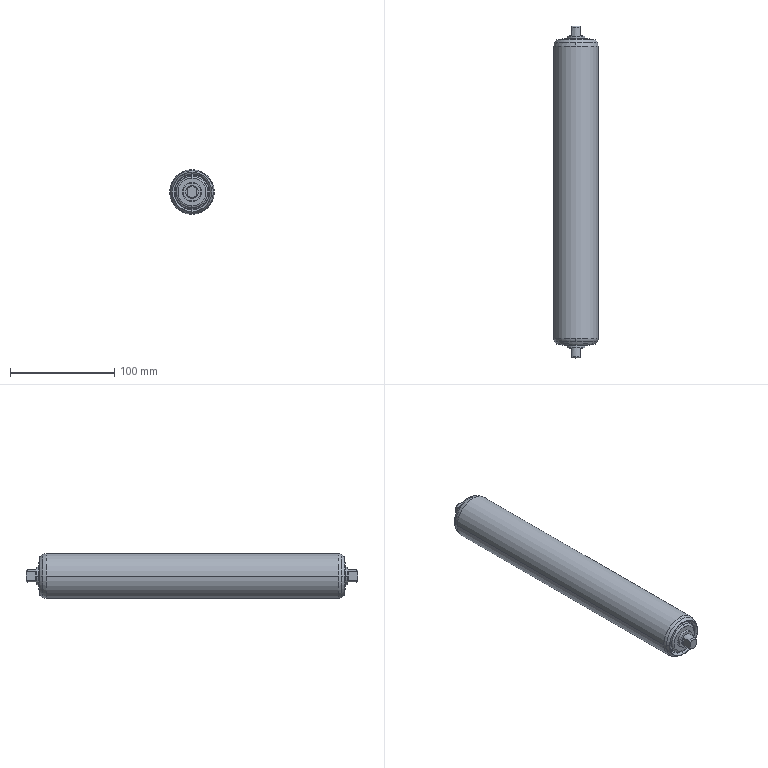Part | STEP file | ROLLER.42.stp | 1 solid | 92 faces | box 43.186 x 318 x 43.662 mm | volume 413616 mm3 | spline 54 | cone 10 | cylinder 10 | plane 10 | torus 8 | commonest cylinder face diameters 12 x2 17 x2 18 x2 30.4 x2 36.3 x2